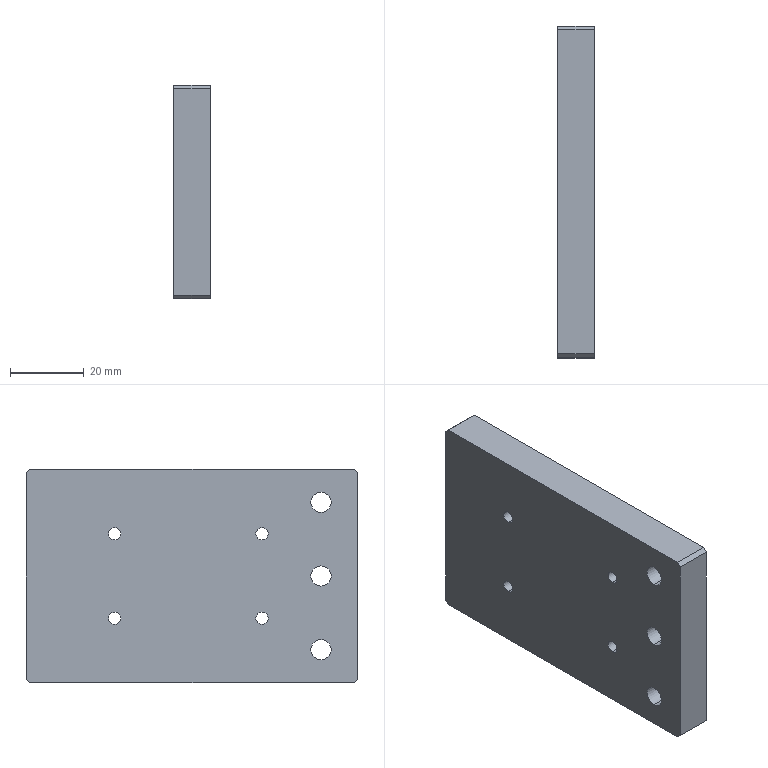Part | SolidWorks | features HoleWzd 2, Chamfer 1, Extrusion 1 | 1 solid | 33 faces | box 10 x 90 x 58 mm | volume 50238 mm3 | cylinder 20 | plane 13 | commonest cylinder face diameters 3.3 x8 5.5 x6 10 x6
STEP:
#1=CARTESIAN_POINT('',(4.6,-35.,25.));
#2=VERTEX_POINT('',#1);
#3=CARTESIAN_POINT('',(4.6,-35.,15.));
#4=VERTEX_POINT('',#3);
#5=CARTESIAN_POINT('',(4.6,-35.,20.));
#6=DIRECTION('',(1.,0.,0.));
#7=DIRECTION('',(0.,0.,-1.));
#8=AXIS2_PLACEMENT_3D('',#5,#6,#7);
#9=CIRCLE('',#8,5.);
#10=EDGE_CURVE('',#2,#4,#9,.T.);
#11=ORIENTED_EDGE('',*,*,#10,.F.);
#12=CARTESIAN_POINT('',(10.,-35.,25.));
#13=VERTEX_POINT('',#12);
#14=CARTESIAN_POINT('',(10.,-35.,25.));
#15=DIRECTION('',(1.,0.,0.));
#16=VECTOR('',#15,1000.);
#17=LINE('',#14,#16);
#18=EDGE_CURVE('',#2,#13,#17,.T.);
#19=ORIENTED_EDGE('',*,*,#18,.T.);
#20=CARTESIAN_POINT('',(10.,-35.,15.));
#21=VERTEX_POINT('',#20);
#22=CARTESIAN_POINT('',(10.,-35.,20.));
#23=DIRECTION('',(1.,0.,0.));
#24=DIRECTION('',(0.,0.,-1.));
#25=AXIS2_PLACEMENT_3D('',#22,#23,#24);
#26=CIRCLE('',#25,5.);
#27=EDGE_CURVE('',#13,#21,#26,.T.);
#28=ORIENTED_EDGE('',*,*,#27,.T.);
#29=CARTESIAN_POINT('',(10.,-35.,15.));
#30=DIRECTION('',(1.,0.,0.));
#31=VECTOR('',#30,1000.);
#32=LINE('',#29,#31);
#33=EDGE_CURVE('',#4,#21,#32,.T.);
#34=ORIENTED_EDGE('',*,*,#33,.F.);
#35=EDGE_LOOP('',(#11,#19,#28,#34));
#36=FACE_OUTER_BOUND('',#35,.T.);
#37=CARTESIAN_POINT('',(10.,-35.,20.));
#38=DIRECTION('',(1.,0.,0.));
#39=DIRECTION('',(0.,0.,-1.));
#40=AXIS2_PLACEMENT_3D('',#37,#38,#39);
#41=CYLINDRICAL_SURFACE('',#40,5.);
#42=ADVANCED_FACE('',(#36),#41,.F.);
#43=CARTESIAN_POINT('',(0.,-35.,22.75));
#44=VERTEX_POINT('',#43);
#45=CARTESIAN_POINT('',(0.,-35.,17.25));
#46=VERTEX_POINT('',#45);
#47=CARTESIAN_POINT('',(0.,-35.,20.));
#48=DIRECTION('',(1.,0.,0.));
#49=DIRECTION('',(0.,0.,-1.));
#50=AXIS2_PLACEMENT_3D('',#47,#48,#49);
#51=CIRCLE('',#50,2.75);
#52=EDGE_CURVE('',#44,#46,#51,.T.);
#53=ORIENTED_EDGE('',*,*,#52,.F.);
#54=CARTESIAN_POINT('',(4.6,-35.,22.75));
#55=VERTEX_POINT('',#54);
#56=CARTESIAN_POINT('',(10.,-35.,22.75));
#57=DIRECTION('',(1.,0.,0.));
#58=VECTOR('',#57,1000.);
#59=LINE('',#56,#58);
#60=EDGE_CURVE('',#44,#55,#59,.T.);
#61=ORIENTED_EDGE('',*,*,#60,.T.);
#62=CARTESIAN_POINT('',(4.6,-35.,17.25));
#63=VERTEX_POINT('',#62);
#64=CARTESIAN_POINT('',(4.6,-35.,20.));
#65=DIRECTION('',(1.,0.,0.));
#66=DIRECTION('',(0.,0.,-1.));
#67=AXIS2_PLACEMENT_3D('',#64,#65,#66);
#68=CIRCLE('',#67,2.75);
#69=EDGE_CURVE('',#55,#63,#68,.T.);
#70=ORIENTED_EDGE('',*,*,#69,.T.);
#71=CARTESIAN_POINT('',(10.,-35.,17.25));
#72=DIRECTION('',(1.,0.,0.));
#73=VECTOR('',#72,1000.);
#74=LINE('',#71,#73);
#75=EDGE_CURVE('',#46,#63,#74,.T.);
#76=ORIENTED_EDGE('',*,*,#75,.F.);
#77=EDGE_LOOP('',(#53,#61,#70,#76));
#78=FACE_OUTER_BOUND('',#77,.T.);
#79=CARTESIAN_POINT('',(10.,-35.,20.));
#80=DIRECTION('',(1.,0.,0.));
#81=DIRECTION('',(0.,0.,-1.));
#82=AXIS2_PLACEMENT_3D('',#79,#80,#81);
#83=CYLINDRICAL_SURFACE('',#82,2.75);
#84=ADVANCED_FACE('',(#78),#83,.F.);
#85=CARTESIAN_POINT('',(4.6,-35.,5.));
#86=VERTEX_POINT('',#85);
#87=CARTESIAN_POINT('',(4.6,-35.,-5.));
#88=VERTEX_POINT('',#87);
#89=CARTESIAN_POINT('',(4.6,-35.,0.));
#90=DIRECTION('',(1.,0.,0.));
#91=DIRECTION('',(0.,0.,-1.));
#92=AXIS2_PLACEMENT_3D('',#89,#90,#91);
#93=CIRCLE('',#92,5.);
#94=EDGE_CURVE('',#86,#88,#93,.T.);
#95=ORIENTED_EDGE('',*,*,#94,.F.);
#96=CARTESIAN_POINT('',(10.,-35.,5.));
#97=VERTEX_POINT('',#96);
#98=CARTESIAN_POINT('',(10.,-35.,5.));
#99=DIRECTION('',(1.,0.,0.));
#100=VECTOR('',#99,1000.);
#101=LINE('',#98,#100);
#102=EDGE_CURVE('',#86,#97,#101,.T.);
#103=ORIENTED_EDGE('',*,*,#102,.T.);
#104=CARTESIAN_POINT('',(10.,-35.,-5.));
#105=VERTEX_POINT('',#104);
#106=CARTESIAN_POINT('',(10.,-35.,0.));
#107=DIRECTION('',(1.,0.,0.));
#108=DIRECTION('',(0.,0.,-1.));
#109=AXIS2_PLACEMENT_3D('',#106,#107,#108);
#110=CIRCLE('',#109,5.);
#111=EDGE_CURVE('',#97,#105,#110,.T.);
#112=ORIENTED_EDGE('',*,*,#111,.T.);
#113=CARTESIAN_POINT('',(10.,-35.,-5.));
#114=DIRECTION('',(1.,0.,0.));
#115=VECTOR('',#114,1000.);
#116=LINE('',#113,#115);
#117=EDGE_CURVE('',#88,#105,#116,.T.);
#118=ORIENTED_EDGE('',*,*,#117,.F.);
#119=EDGE_LOOP('',(#95,#103,#112,#118));
#120=FACE_OUTER_BOUND('',#119,.T.);
#121=CARTESIAN_POINT('',(10.,-35.,0.));
#122=DIRECTION('',(1.,0.,0.));
#123=DIRECTION('',(0.,0.,-1.));
#124=AXIS2_PLACEMENT_3D('',#121,#122,#123);
#125=CYLINDRICAL_SURFACE('',#124,5.);
#126=ADVANCED_FACE('',(#120),#125,.F.);
#127=CARTESIAN_POINT('',(0.,-35.,2.75));
#128=VERTEX_POINT('',#127);
#129=CARTESIAN_POINT('',(0.,-35.,-2.75));
#130=VERTEX_POINT('',#129);
#131=CARTESIAN_POINT('',(0.,-35.,0.));
#132=DIRECTION('',(1.,0.,0.));
#133=DIRECTION('',(0.,0.,-1.));
#134=AXIS2_PLACEMENT_3D('',#131,#132,#133);
#135=CIRCLE('',#134,2.75);
#136=EDGE_CURVE('',#128,#130,#135,.T.);
#137=ORIENTED_EDGE('',*,*,#136,.F.);
#138=CARTESIAN_POINT('',(4.6,-35.,2.75));
#139=VERTEX_POINT('',#138);
#140=CARTESIAN_POINT('',(10.,-35.,2.75));
#141=DIRECTION('',(1.,0.,0.));
#142=VECTOR('',#141,1000.);
#143=LINE('',#140,#142);
#144=EDGE_CURVE('',#128,#139,#143,.T.);
#145=ORIENTED_EDGE('',*,*,#144,.T.);
#146=CARTESIAN_POINT('',(4.6,-35.,-2.75));
#147=VERTEX_POINT('',#146);
#148=CARTESIAN_POINT('',(4.6,-35.,0.));
#149=DIRECTION('',(1.,0.,0.));
#150=DIRECTION('',(0.,0.,-1.));
#151=AXIS2_PLACEMENT_3D('',#148,#149,#150);
#152=CIRCLE('',#151,2.75);
#153=EDGE_CURVE('',#139,#147,#152,.T.);
#154=ORIENTED_EDGE('',*,*,#153,.T.);
#155=CARTESIAN_POINT('',(10.,-35.,-2.75));
#156=DIRECTION('',(1.,0.,0.));
#157=VECTOR('',#156,1000.);
#158=LINE('',#155,#157);
#159=EDGE_CURVE('',#130,#147,#158,.T.);
#160=ORIENTED_EDGE('',*,*,#159,.F.);
#161=EDGE_LOOP('',(#137,#145,#154,#160));
#162=FACE_OUTER_BOUND('',#161,.T.);
#163=CARTESIAN_POINT('',(10.,-35.,0.));
#164=DIRECTION('',(1.,0.,0.));
#165=DIRECTION('',(0.,0.,-1.));
#166=AXIS2_PLACEMENT_3D('',#163,#164,#165);
#167=CYLINDRICAL_SURFACE('',#166,2.75);
#168=ADVANCED_FACE('',(#162),#167,.F.);
#169=CARTESIAN_POINT('',(4.6,-35.,-15.));
#170=VERTEX_POINT('',#169);
#171=CARTESIAN_POINT('',(4.6,-35.,-25.));
#172=VERTEX_POINT('',#171);
#173=CARTESIAN_POINT('',(4.6,-35.,-20.));
#174=DIRECTION('',(1.,0.,0.));
#175=DIRECTION('',(0.,0.,-1.));
#176=AXIS2_PLACEMENT_3D('',#173,#174,#175);
#177=CIRCLE('',#176,5.);
#178=EDGE_CURVE('',#170,#172,#177,.T.);
#179=ORIENTED_EDGE('',*,*,#178,.F.);
#180=CARTESIAN_POINT('',(10.,-35.,-15.));
#181=VERTEX_POINT('',#180);
#182=CARTESIAN_POINT('',(10.,-35.,-15.));
#183=DIRECTION('',(1.,0.,0.));
#184=VECTOR('',#183,1000.);
#185=LINE('',#182,#184);
#186=EDGE_CURVE('',#170,#181,#185,.T.);
#187=ORIENTED_EDGE('',*,*,#186,.T.);
#188=CARTESIAN_POINT('',(10.,-35.,-25.));
#189=VERTEX_POINT('',#188);
#190=CARTESIAN_POINT('',(10.,-35.,-20.));
#191=DIRECTION('',(1.,0.,0.));
#192=DIRECTION('',(0.,0.,-1.));
#193=AXIS2_PLACEMENT_3D('',#190,#191,#192);
#194=CIRCLE('',#193,5.);
#195=EDGE_CURVE('',#181,#189,#194,.T.);
#196=ORIENTED_EDGE('',*,*,#195,.T.);
#197=CARTESIAN_POINT('',(10.,-35.,-25.));
#198=DIRECTION('',(1.,0.,0.));
#199=VECTOR('',#198,1000.);
#200=LINE('',#197,#199);
#201=EDGE_CURVE('',#172,#189,#200,.T.);
#202=ORIENTED_EDGE('',*,*,#201,.F.);
#203=EDGE_LOOP('',(#179,#187,#196,#202));
#204=FACE_OUTER_BOUND('',#203,.T.);
#205=CARTESIAN_POINT('',(10.,-35.,-20.));
#206=DIRECTION('',(1.,0.,0.));
#207=DIRECTION('',(0.,0.,-1.));
#208=AXIS2_PLACEMENT_3D('',#205,#206,#207);
#209=CYLINDRICAL_SURFACE('',#208,5.);
#210=ADVANCED_FACE('',(#204),#209,.F.);
#211=CARTESIAN_POINT('',(0.,-35.,-17.25));
#212=VERTEX_POINT('',#211);
#213=CARTESIAN_POINT('',(0.,-35.,-22.75));
#214=VERTEX_POINT('',#213);
#215=CARTESIAN_POINT('',(0.,-35.,-20.));
#216=DIRECTION('',(1.,0.,0.));
#217=DIRECTION('',(0.,0.,-1.));
#218=AXIS2_PLACEMENT_3D('',#215,#216,#217);
#219=CIRCLE('',#218,2.75);
#220=EDGE_CURVE('',#212,#214,#219,.T.);
#221=ORIENTED_EDGE('',*,*,#220,.F.);
#222=CARTESIAN_POINT('',(4.6,-35.,-17.25));
#223=VERTEX_POINT('',#222);
#224=CARTESIAN_POINT('',(10.,-35.,-17.25));
#225=DIRECTION('',(1.,0.,0.));
#226=VECTOR('',#225,1000.);
#227=LINE('',#224,#226);
#228=EDGE_CURVE('',#212,#223,#227,.T.);
#229=ORIENTED_EDGE('',*,*,#228,.T.);
#230=CARTESIAN_POINT('',(4.6,-35.,-22.75));
#231=VERTEX_POINT('',#230);
#232=CARTESIAN_POINT('',(4.6,-35.,-20.));
#233=DIRECTION('',(1.,0.,0.));
#234=DIRECTION('',(0.,0.,-1.));
#235=AXIS2_PLACEMENT_3D('',#232,#233,#234);
#236=CIRCLE('',#235,2.75);
#237=EDGE_CURVE('',#223,#231,#236,.T.);
#238=ORIENTED_EDGE('',*,*,#237,.T.);
#239=CARTESIAN_POINT('',(10.,-35.,-22.75));
#240=DIRECTION('',(1.,0.,0.));
#241=VECTOR('',#240,1000.);
#242=LINE('',#239,#241);
#243=EDGE_CURVE('',#214,#231,#242,.T.);
#244=ORIENTED_EDGE('',*,*,#243,.F.);
#245=EDGE_LOOP('',(#221,#229,#238,#244));
#246=FACE_OUTER_BOUND('',#245,.T.);
#247=CARTESIAN_POINT('',(10.,-35.,-20.));
#248=DIRECTION('',(1.,0.,0.));
#249=DIRECTION('',(0.,0.,-1.));
#250=AXIS2_PLACEMENT_3D('',#247,#248,#249);
#251=CYLINDRICAL_SURFACE('',#250,2.75);
#252=ADVANCED_FACE('',(#246),#251,.F.);
#253=CARTESIAN_POINT('',(0.,21.,13.15));
#254=VERTEX_POINT('',#253);
#255=CARTESIAN_POINT('',(0.,21.,9.85));
#256=VERTEX_POINT('',#255);
#257=CARTESIAN_POINT('',(0.,21.,11.5));
#258=DIRECTION('',(1.,0.,0.));
#259=DIRECTION('',(0.,0.,-1.));
#260=AXIS2_PLACEMENT_3D('',#257,#258,#259);
#261=CIRCLE('',#260,1.65);
#262=EDGE_CURVE('',#254,#256,#261,.T.);
#263=ORIENTED_EDGE('',*,*,#262,.F.);
#264=CARTESIAN_POINT('',(10.,21.,13.15));
#265=VERTEX_POINT('',#264);
#266=CARTESIAN_POINT('',(10.,21.,13.15));
#267=DIRECTION('',(1.,0.,0.));
#268=VECTOR('',#267,1000.);
#269=LINE('',#266,#268);
#270=EDGE_CURVE('',#254,#265,#269,.T.);
#271=ORIENTED_EDGE('',*,*,#270,.T.);
#272=CARTESIAN_POINT('',(10.,21.,9.85));
#273=VERTEX_POINT('',#272);
#274=CARTESIAN_POINT('',(10.,21.,11.5));
#275=DIRECTION('',(1.,0.,0.));
#276=DIRECTION('',(0.,0.,-1.));
#277=AXIS2_PLACEMENT_3D('',#274,#275,#276);
#278=CIRCLE('',#277,1.65);
#279=EDGE_CURVE('',#265,#273,#278,.T.);
#280=ORIENTED_EDGE('',*,*,#279,.T.);
#281=CARTESIAN_POINT('',(10.,21.,9.85));
#282=DIRECTION('',(1.,0.,0.));
#283=VECTOR('',#282,1000.);
#284=LINE('',#281,#283);
#285=EDGE_CURVE('',#256,#273,#284,.T.);
#286=ORIENTED_EDGE('',*,*,#285,.F.);
#287=EDGE_LOOP('',(#263,#271,#280,#286));
#288=FACE_OUTER_BOUND('',#287,.T.);
#289=CARTESIAN_POINT('',(10.,21.,11.5));
#290=DIRECTION('',(1.,0.,0.));
#291=DIRECTION('',(0.,0.,-1.));
#292=AXIS2_PLACEMENT_3D('',#289,#290,#291);
#293=CYLINDRICAL_SURFACE('',#292,1.65);
#294=ADVANCED_FACE('',(#288),#293,.F.);
#295=CARTESIAN_POINT('',(0.,21.,-9.85));
#296=VERTEX_POINT('',#295);
#297=CARTESIAN_POINT('',(0.,21.,-13.15));
#298=VERTEX_POINT('',#297);
#299=CARTESIAN_POINT('',(0.,21.,-11.5));
#300=DIRECTION('',(1.,0.,0.));
#301=DIRECTION('',(0.,0.,-1.));
#302=AXIS2_PLACEMENT_3D('',#299,#300,#301);
#303=CIRCLE('',#302,1.65);
#304=EDGE_CURVE('',#296,#298,#303,.T.);
#305=ORIENTED_EDGE('',*,*,#304,.F.);
#306=CARTESIAN_POINT('',(10.,21.,-9.85));
#307=VERTEX_POINT('',#306);
#308=CARTESIAN_POINT('',(10.,21.,-9.85));
#309=DIRECTION('',(1.,0.,0.));
#310=VECTOR('',#309,1000.);
#311=LINE('',#308,#310);
#312=EDGE_CURVE('',#296,#307,#311,.T.);
#313=ORIENTED_EDGE('',*,*,#312,.T.);
#314=CARTESIAN_POINT('',(10.,21.,-13.15));
#315=VERTEX_POINT('',#314);
#316=CARTESIAN_POINT('',(10.,21.,-11.5));
#317=DIRECTION('',(1.,0.,0.));
#318=DIRECTION('',(0.,0.,-1.));
#319=AXIS2_PLACEMENT_3D('',#316,#317,#318);
#320=CIRCLE('',#319,1.65);
#321=EDGE_CURVE('',#307,#315,#320,.T.);
#322=ORIENTED_EDGE('',*,*,#321,.T.);
#323=CARTESIAN_POINT('',(10.,21.,-13.15));
#324=DIRECTION('',(1.,0.,0.));
#325=VECTOR('',#324,1000.);
#326=LINE('',#323,#325);
#327=EDGE_CURVE('',#298,#315,#326,.T.);
#328=ORIENTED_EDGE('',*,*,#327,.F.);
#329=EDGE_LOOP('',(#305,#313,#322,#328));
#330=FACE_OUTER_BOUND('',#329,.T.);
#331=CARTESIAN_POINT('',(10.,21.,-11.5));
#332=DIRECTION('',(1.,0.,0.));
#333=DIRECTION('',(0.,0.,-1.));
#334=AXIS2_PLACEMENT_3D('',#331,#332,#333);
#335=CYLINDRICAL_SURFACE('',#334,1.65);
#336=ADVANCED_FACE('',(#330),#335,.F.);
#337=CARTESIAN_POINT('',(0.,-19.,13.15));
#338=VERTEX_POINT('',#337);
#339=CARTESIAN_POINT('',(0.,-19.,9.85));
#340=VERTEX_POINT('',#339);
#341=CARTESIAN_POINT('',(0.,-19.,11.5));
#342=DIRECTION('',(1.,0.,0.));
#343=DIRECTION('',(0.,0.,-1.));
#344=AXIS2_PLACEMENT_3D('',#341,#342,#343);
#345=CIRCLE('',#344,1.65);
#346=EDGE_CURVE('',#338,#340,#345,.T.);
#347=ORIENTED_EDGE('',*,*,#346,.F.);
#348=CARTESIAN_POINT('',(10.,-19.,13.15));
#349=VERTEX_POINT('',#348);
#350=CARTESIAN_POINT('',(10.,-19.,13.15));
#351=DIRECTION('',(1.,0.,0.));
#352=VECTOR('',#351,1000.);
#353=LINE('',#350,#352);
#354=EDGE_CURVE('',#338,#349,#353,.T.);
#355=ORIENTED_EDGE('',*,*,#354,.T.);
#356=CARTESIAN_POINT('',(10.,-19.,9.85));
#357=VERTEX_POINT('',#356);
#358=CARTESIAN_POINT('',(10.,-19.,11.5));
#359=DIRECTION('',(1.,0.,0.));
#360=DIRECTION('',(0.,0.,-1.));
#361=AXIS2_PLACEMENT_3D('',#358,#359,#360);
#362=CIRCLE('',#361,1.65);
#363=EDGE_CURVE('',#349,#357,#362,.T.);
#364=ORIENTED_EDGE('',*,*,#363,.T.);
#365=CARTESIAN_POINT('',(10.,-19.,9.85));
#366=DIRECTION('',(1.,0.,0.));
#367=VECTOR('',#366,1000.);
#368=LINE('',#365,#367);
#369=EDGE_CURVE('',#340,#357,#368,.T.);
#370=ORIENTED_EDGE('',*,*,#369,.F.);
#371=EDGE_LOOP('',(#347,#355,#364,#370));
#372=FACE_OUTER_BOUND('',#371,.T.);
#373=CARTESIAN_POINT('',(10.,-19.,11.5));
#374=DIRECTION('',(1.,0.,0.));
#375=DIRECTION('',(0.,0.,-1.));
#376=AXIS2_PLACEMENT_3D('',#373,#374,#375);
#377=CYLINDRICAL_SURFACE('',#376,1.65);
#378=ADVANCED_FACE('',(#372),#377,.F.);
#379=CARTESIAN_POINT('',(0.,-19.,-9.85));
#380=VERTEX_POINT('',#379);
#381=CARTESIAN_POINT('',(0.,-19.,-13.15));
#382=VERTEX_POINT('',#381);
#383=CARTESIAN_POINT('',(0.,-19.,-11.5));
#384=DIRECTION('',(1.,0.,0.));
#385=DIRECTION('',(0.,0.,-1.));
#386=AXIS2_PLACEMENT_3D('',#383,#384,#385);
#387=CIRCLE('',#386,1.65);
#388=EDGE_CURVE('',#380,#382,#387,.T.);
#389=ORIENTED_EDGE('',*,*,#388,.F.);
#390=CARTESIAN_POINT('',(10.,-19.,-9.85));
#391=VERTEX_POINT('',#390);
#392=CARTESIAN_POINT('',(10.,-19.,-9.85));
#393=DIRECTION('',(1.,0.,0.));
#394=VECTOR('',#393,1000.);
#395=LINE('',#392,#394);
#396=EDGE_CURVE('',#380,#391,#395,.T.);
#397=ORIENTED_EDGE('',*,*,#396,.T.);
#398=CARTESIAN_POINT('',(10.,-19.,-13.15));
#399=VERTEX_POINT('',#398);
#400=CARTESIAN_POINT('',(10.,-19.,-11.5));
#401=DIRECTION('',(1.,0.,0.));
#402=DIRECTION('',(0.,0.,-1.));
#403=AXIS2_PLACEMENT_3D('',#400,#401,#402);
#404=CIRCLE('',#403,1.65);
#405=EDGE_CURVE('',#391,#399,#404,.T.);
#406=ORIENTED_EDGE('',*,*,#405,.T.);
#407=CARTESIAN_POINT('',(10.,-19.,-13.15));
#408=DIRECTION('',(1.,0.,0.));
#409=VECTOR('',#408,1000.);
#410=LINE('',#407,#409);
#411=EDGE_CURVE('',#382,#399,#410,.T.);
#412=ORIENTED_EDGE('',*,*,#411,.F.);
#413=EDGE_LOOP('',(#389,#397,#406,#412));
#414=FACE_OUTER_BOUND('',#413,.T.);
#415=CARTESIAN_POINT('',(10.,-19.,-11.5));
#416=DIRECTION('',(1.,0.,0.));
#417=DIRECTION('',(0.,0.,-1.));
#418=AXIS2_PLACEMENT_3D('',#415,#416,#417);
#419=CYLINDRICAL_SURFACE('',#418,1.65);
#420=ADVANCED_FACE('',(#414),#419,.F.);
#421=CARTESIAN_POINT('',(10.,-44.,-29.));
#422=VERTEX_POINT('',#421);
#423=CARTESIAN_POINT('',(10.,44.,-29.));
#424=VERTEX_POINT('',#423);
#425=CARTESIAN_POINT('',(10.,45.,-29.));
#426=DIRECTION('',(0.,1.,0.));
#427=VECTOR('',#426,1000.);
#428=LINE('',#425,#427);
#429=EDGE_CURVE('',#422,#424,#428,.T.);
#430=ORIENTED_EDGE('',*,*,#429,.F.);
#431=CARTESIAN_POINT('',(0.,-44.,-29.));
#432=VERTEX_POINT('',#431);
#433=CARTESIAN_POINT('',(10.,-44.,-29.));
#434=DIRECTION('',(-1.,0.,0.));
#435=VECTOR('',#434,1000.);
#436=LINE('',#433,#435);
#437=EDGE_CURVE('',#422,#432,#436,.T.);
#438=ORIENTED_EDGE('',*,*,#437,.T.);
#439=CARTESIAN_POINT('',(0.,44.,-29.));
#440=VERTEX_POINT('',#439);
#441=CARTESIAN_POINT('',(0.,45.,-29.));
#442=DIRECTION('',(0.,1.,0.));
#443=VECTOR('',#442,1000.);
#444=LINE('',#441,#443);
#445=EDGE_CURVE('',#432,#440,#444,.T.);
#446=ORIENTED_EDGE('',*,*,#445,.T.);
#447=CARTESIAN_POINT('',(10.,44.,-29.));
#448=DIRECTION('',(1.,0.,0.));
#449=VECTOR('',#448,1000.);
#450=LINE('',#447,#449);
#451=EDGE_CURVE('',#440,#424,#450,.T.);
#452=ORIENTED_EDGE('',*,*,#451,.T.);
#453=EDGE_LOOP('',(#430,#438,#446,#452));
#454=FACE_OUTER_BOUND('',#453,.T.);
#455=CARTESIAN_POINT('',(10.,45.,-29.));
#456=DIRECTION('',(0.,0.,1.));
#457=DIRECTION('',(0.,-1.,0.));
#458=AXIS2_PLACEMENT_3D('',#455,#456,#457);
#459=PLANE('',#458);
#460=ADVANCED_FACE('',(#454),#459,.F.);
#461=CARTESIAN_POINT('',(10.,45.,-28.));
#462=VERTEX_POINT('',#461);
#463=CARTESIAN_POINT('',(10.,45.,28.));
#464=VERTEX_POINT('',#463);
#465=CARTESIAN_POINT('',(10.,45.,29.));
#466=DIRECTION('',(0.,0.,1.));
#467=VECTOR('',#466,1000.);
#468=LINE('',#465,#467);
#469=EDGE_CURVE('',#462,#464,#468,.T.);
#470=ORIENTED_EDGE('',*,*,#469,.F.);
#471=CARTESIAN_POINT('',(0.,45.,-28.));
#472=VERTEX_POINT('',#471);
#473=CARTESIAN_POINT('',(10.,45.,-28.));
#474=DIRECTION('',(-1.,0.,0.));
#475=VECTOR('',#474,1000.);
#476=LINE('',#473,#475);
#477=EDGE_CURVE('',#462,#472,#476,.T.);
#478=ORIENTED_EDGE('',*,*,#477,.T.);
#479=CARTESIAN_POINT('',(0.,45.,28.));
#480=VERTEX_POINT('',#479);
#481=CARTESIAN_POINT('',(0.,45.,29.));
#482=DIRECTION('',(0.,0.,1.));
#483=VECTOR('',#482,1000.);
#484=LINE('',#481,#483);
#485=EDGE_CURVE('',#472,#480,#484,.T.);
#486=ORIENTED_EDGE('',*,*,#485,.T.);
#487=CARTESIAN_POINT('',(10.,45.,28.));
#488=DIRECTION('',(1.,0.,0.));
#489=VECTOR('',#488,1000.);
#490=LINE('',#487,#489);
#491=EDGE_CURVE('',#480,#464,#490,.T.);
#492=ORIENTED_EDGE('',*,*,#491,.T.);
#493=EDGE_LOOP('',(#470,#478,#486,#492));
#494=FACE_OUTER_BOUND('',#493,.T.);
#495=CARTESIAN_POINT('',(10.,45.,29.));
#496=DIRECTION('',(0.,-1.,0.));
#497=DIRECTION('',(0.,0.,-1.));
#498=AXIS2_PLACEMENT_3D('',#495,#496,#497);
#499=PLANE('',#498);
#500=ADVANCED_FACE('',(#494),#499,.F.);
#501=CARTESIAN_POINT('',(0.,44.,29.));
#502=VERTEX_POINT('',#501);
#503=CARTESIAN_POINT('',(0.,-44.,29.));
#504=VERTEX_POINT('',#503);
#505=CARTESIAN_POINT('',(0.,45.,29.));
#506=DIRECTION('',(0.,-1.,0.));
#507=VECTOR('',#506,1000.);
#508=LINE('',#505,#507);
#509=EDGE_CURVE('',#502,#504,#508,.T.);
#510=ORIENTED_EDGE('',*,*,#509,.T.);
#511=CARTESIAN_POINT('',(10.,-44.,29.));
#512=VERTEX_POINT('',#511);
#513=CARTESIAN_POINT('',(10.,-44.,29.));
#514=DIRECTION('',(1.,0.,0.));
#515=VECTOR('',#514,1000.);
#516=LINE('',#513,#515);
#517=EDGE_CURVE('',#504,#512,#516,.T.);
#518=ORIENTED_EDGE('',*,*,#517,.T.);
#519=CARTESIAN_POINT('',(10.,44.,29.));
#520=VERTEX_POINT('',#519);
#521=CARTESIAN_POINT('',(10.,45.,29.));
#522=DIRECTION('',(0.,-1.,0.));
#523=VECTOR('',#522,1000.);
#524=LINE('',#521,#523);
#525=EDGE_CURVE('',#520,#512,#524,.T.);
#526=ORIENTED_EDGE('',*,*,#525,.F.);
#527=CARTESIAN_POINT('',(10.,44.,29.));
#528=DIRECTION('',(-1.,0.,0.));
#529=VECTOR('',#528,1000.);
#530=LINE('',#527,#529);
#531=EDGE_CURVE('',#520,#502,#530,.T.);
#532=ORIENTED_EDGE('',*,*,#531,.T.);
#533=EDGE_LOOP('',(#510,#518,#526,#532));
#534=FACE_OUTER_BOUND('',#533,.T.);
#535=CARTESIAN_POINT('',(10.,45.,29.));
#536=DIRECTION('',(0.,0.,-1.));
#537=DIRECTION('',(0.,1.,0.));
#538=AXIS2_PLACEMENT_3D('',#535,#536,#537);
#539=PLANE('',#538);
#540=ADVANCED_FACE('',(#534),#539,.F.);
#541=CARTESIAN_POINT('',(0.,-45.,28.));
#542=VERTEX_POINT('',#541);
#543=CARTESIAN_POINT('',(0.,-45.,-28.));
#544=VERTEX_POINT('',#543);
#545=CARTESIAN_POINT('',(0.,-45.,29.));
#546=DIRECTION('',(0.,0.,-1.));
#547=VECTOR('',#546,1000.);
#548=LINE('',#545,#547);
#549=EDGE_CURVE('',#542,#544,#548,.T.);
#550=ORIENTED_EDGE('',*,*,#549,.T.);
#551=CARTESIAN_POINT('',(10.,-45.,-28.));
#552=VERTEX_POINT('',#551);
#553=CARTESIAN_POINT('',(10.,-45.,-28.));
#554=DIRECTION('',(1.,0.,0.));
#555=VECTOR('',#554,1000.);
#556=LINE('',#553,#555);
#557=EDGE_CURVE('',#544,#552,#556,.T.);
#558=ORIENTED_EDGE('',*,*,#557,.T.);
#559=CARTESIAN_POINT('',(10.,-45.,28.));
#560=VERTEX_POINT('',#559);
#561=CARTESIAN_POINT('',(10.,-45.,29.));
#562=DIRECTION('',(0.,0.,-1.));
#563=VECTOR('',#562,1000.);
#564=LINE('',#561,#563);
#565=EDGE_CURVE('',#560,#552,#564,.T.);
#566=ORIENTED_EDGE('',*,*,#565,.F.);
#567=CARTESIAN_POINT('',(10.,-45.,28.));
#568=DIRECTION('',(-1.,0.,0.));
#569=VECTOR('',#568,1000.);
#570=LINE('',#567,#569);
#571=EDGE_CURVE('',#560,#542,#570,.T.);
#572=ORIENTED_EDGE('',*,*,#571,.T.);
#573=EDGE_LOOP('',(#550,#558,#566,#572));
#574=FACE_OUTER_BOUND('',#573,.T.);
#575=CARTESIAN_POINT('',(10.,-45.,29.));
#576=DIRECTION('',(0.,1.,0.));
#577=DIRECTION('',(0.,0.,1.));
#578=AXIS2_PLACEMENT_3D('',#575,#576,#577);
#579=PLANE('',#578);
#580=ADVANCED_FACE('',(#574),#579,.F.);
#581=CARTESIAN_POINT('',(10.,-35.,20.));
#582=DIRECTION('',(1.,0.,0.));
#583=DIRECTION('',(0.,0.,-1.));
#584=AXIS2_PLACEMENT_3D('',#581,#582,#583);
#585=CIRCLE('',#584,5.);
#586=EDGE_CURVE('',#21,#13,#585,.T.);
#587=ORIENTED_EDGE('',*,*,#586,.F.);
#588=ORIENTED_EDGE('',*,*,#27,.F.);
#589=EDGE_LOOP('',(#587,#588));
#590=FACE_BOUND('',#589,.T.);
#591=CARTESIAN_POINT('',(10.,-35.,0.));
#592=DIRECTION('',(1.,0.,0.));
#593=DIRECTION('',(0.,0.,-1.));
#594=AXIS2_PLACEMENT_3D('',#591,#592,#593);
#595=CIRCLE('',#594,5.);
#596=EDGE_CURVE('',#105,#97,#595,.T.);
#597=ORIENTED_EDGE('',*,*,#596,.F.);
#598=ORIENTED_EDGE('',*,*,#111,.F.);
#599=EDGE_LOOP('',(#597,#598));
#600=FACE_BOUND('',#599,.T.);
#601=CARTESIAN_POINT('',(10.,-35.,-20.));
#602=DIRECTION('',(1.,0.,0.));
#603=DIRECTION('',(0.,0.,-1.));
#604=AXIS2_PLACEMENT_3D('',#601,#602,#603);
#605=CIRCLE('',#604,5.);
#606=EDGE_CURVE('',#189,#181,#605,.T.);
#607=ORIENTED_EDGE('',*,*,#606,.F.);
#608=ORIENTED_EDGE('',*,*,#195,.F.);
#609=EDGE_LOOP('',(#607,#608));
#610=FACE_BOUND('',#609,.T.);
#611=CARTESIAN_POINT('',(10.,21.,11.5));
#612=DIRECTION('',(1.,0.,0.));
#613=DIRECTION('',(0.,0.,-1.));
#614=AXIS2_PLACEMENT_3D('',#611,#612,#613);
#615=CIRCLE('',#614,1.65);
#616=EDGE_CURVE('',#273,#265,#615,.T.);
#617=ORIENTED_EDGE('',*,*,#616,.F.);
#618=ORIENTED_EDGE('',*,*,#279,.F.);
#619=EDGE_LOOP('',(#617,#618));
#620=FACE_BOUND('',#619,.T.);
#621=CARTESIAN_POINT('',(10.,21.,-11.5));
#622=DIRECTION('',(1.,0.,0.));
#623=DIRECTION('',(0.,0.,-1.));
#624=AXIS2_PLACEMENT_3D('',#621,#622,#623);
#625=CIRCLE('',#624,1.65);
#626=EDGE_CURVE('',#315,#307,#625,.T.);
#627=ORIENTED_EDGE('',*,*,#626,.F.);
#628=ORIENTED_EDGE('',*,*,#321,.F.);
#629=EDGE_LOOP('',(#627,#628));
#630=FACE_BOUND('',#629,.T.);
#631=CARTESIAN_POINT('',(10.,-19.,11.5));
#632=DIRECTION('',(1.,0.,0.));
#633=DIRECTION('',(0.,0.,-1.));
#634=AXIS2_PLACEMENT_3D('',#631,#632,#633);
#635=CIRCLE('',#634,1.65);
#636=EDGE_CURVE('',#357,#349,#635,.T.);
#637=ORIENTED_EDGE('',*,*,#636,.F.);
#638=ORIENTED_EDGE('',*,*,#363,.F.);
#639=EDGE_LOOP('',(#637,#638));
#640=FACE_BOUND('',#639,.T.);
#641=CARTESIAN_POINT('',(10.,-19.,-11.5));
#642=DIRECTION('',(1.,0.,0.));
#643=DIRECTION('',(0.,0.,-1.));
#644=AXIS2_PLACEMENT_3D('',#641,#642,#643);
#645=CIRCLE('',#644,1.65);
#646=EDGE_CURVE('',#399,#391,#645,.T.);
#647=ORIENTED_EDGE('',*,*,#646,.F.);
#648=ORIENTED_EDGE('',*,*,#405,.F.);
#649=EDGE_LOOP('',(#647,#648));
#650=FACE_BOUND('',#649,.T.);
#651=ORIENTED_EDGE('',*,*,#565,.T.);
#652=CARTESIAN_POINT('',(10.,-36.5,-36.5));
#653=DIRECTION('',(0.,0.7071,-0.7071));
#654=VECTOR('',#653,1000.);
#655=LINE('',#652,#654);
#656=EDGE_CURVE('',#552,#422,#655,.T.);
#657=ORIENTED_EDGE('',*,*,#656,.T.);
#658=ORIENTED_EDGE('',*,*,#429,.T.);
#659=CARTESIAN_POINT('',(10.,36.5,-36.5));
#660=DIRECTION('',(0.,0.7071,0.7071));
#661=VECTOR('',#660,1000.);
#662=LINE('',#659,#661);
#663=EDGE_CURVE('',#424,#462,#662,.T.);
#664=ORIENTED_EDGE('',*,*,#663,.T.);
#665=ORIENTED_EDGE('',*,*,#469,.T.);
#666=CARTESIAN_POINT('',(10.,36.5,36.5));
#667=DIRECTION('',(0.,-0.7071,0.7071));
#668=VECTOR('',#667,1000.);
#669=LINE('',#666,#668);
#670=EDGE_CURVE('',#464,#520,#669,.T.);
#671=ORIENTED_EDGE('',*,*,#670,.T.);
#672=ORIENTED_EDGE('',*,*,#525,.T.);
#673=CARTESIAN_POINT('',(10.,-36.5,36.5));
#674=DIRECTION('',(0.,-0.7071,-0.7071));
#675=VECTOR('',#674,1000.);
#676=LINE('',#673,#675);
#677=EDGE_CURVE('',#512,#560,#676,.T.);
#678=ORIENTED_EDGE('',*,*,#677,.T.);
#679=EDGE_LOOP('',(#651,#657,#658,#664,#665,#671,#672,#678));
#680=FACE_OUTER_BOUND('',#679,.T.);
#681=CARTESIAN_POINT('',(10.,0.,0.));
#682=DIRECTION('',(1.,0.,0.));
#683=DIRECTION('',(0.,0.,-1.));
#684=AXIS2_PLACEMENT_3D('',#681,#682,#683);
#685=PLANE('',#684);
#686=ADVANCED_FACE('',(#590,#600,#610,#620,#630,#640,#650,#680),#685,.T.);
#687=CARTESIAN_POINT('',(0.,-35.,20.));
#688=DIRECTION('',(1.,0.,0.));
#689=DIRECTION('',(0.,0.,-1.));
#690=AXIS2_PLACEMENT_3D('',#687,#688,#689);
#691=CIRCLE('',#690,2.75);
#692=EDGE_CURVE('',#46,#44,#691,.T.);
#693=ORIENTED_EDGE('',*,*,#692,.T.);
#694=ORIENTED_EDGE('',*,*,#52,.T.);
#695=EDGE_LOOP('',(#693,#694));
#696=FACE_BOUND('',#695,.T.);
#697=CARTESIAN_POINT('',(0.,-35.,0.));
#698=DIRECTION('',(1.,0.,0.));
#699=DIRECTION('',(0.,0.,-1.));
#700=AXIS2_PLACEMENT_3D('',#697,#698,#699);
#701=CIRCLE('',#700,2.75);
#702=EDGE_CURVE('',#130,#128,#701,.T.);
#703=ORIENTED_EDGE('',*,*,#702,.T.);
#704=ORIENTED_EDGE('',*,*,#136,.T.);
#705=EDGE_LOOP('',(#703,#704));
#706=FACE_BOUND('',#705,.T.);
#707=CARTESIAN_POINT('',(0.,-35.,-20.));
#708=DIRECTION('',(1.,0.,0.));
#709=DIRECTION('',(0.,0.,-1.));
#710=AXIS2_PLACEMENT_3D('',#707,#708,#709);
#711=CIRCLE('',#710,2.75);
#712=EDGE_CURVE('',#214,#212,#711,.T.);
#713=ORIENTED_EDGE('',*,*,#712,.T.);
#714=ORIENTED_EDGE('',*,*,#220,.T.);
#715=EDGE_LOOP('',(#713,#714));
#716=FACE_BOUND('',#715,.T.);
#717=CARTESIAN_POINT('',(0.,21.,11.5));
#718=DIRECTION('',(1.,0.,0.));
#719=DIRECTION('',(0.,0.,-1.));
#720=AXIS2_PLACEMENT_3D('',#717,#718,#719);
#721=CIRCLE('',#720,1.65);
#722=EDGE_CURVE('',#256,#254,#721,.T.);
#723=ORIENTED_EDGE('',*,*,#722,.T.);
#724=ORIENTED_EDGE('',*,*,#262,.T.);
#725=EDGE_LOOP('',(#723,#724));
#726=FACE_BOUND('',#725,.T.);
#727=CARTESIAN_POINT('',(0.,21.,-11.5));
#728=DIRECTION('',(1.,0.,0.));
#729=DIRECTION('',(0.,0.,-1.));
#730=AXIS2_PLACEMENT_3D('',#727,#728,#729);
#731=CIRCLE('',#730,1.65);
#732=EDGE_CURVE('',#298,#296,#731,.T.);
#733=ORIENTED_EDGE('',*,*,#732,.T.);
#734=ORIENTED_EDGE('',*,*,#304,.T.);
#735=EDGE_LOOP('',(#733,#734));
#736=FACE_BOUND('',#735,.T.);
#737=CARTESIAN_POINT('',(0.,-19.,11.5));
#738=DIRECTION('',(1.,0.,0.));
#739=DIRECTION('',(0.,0.,-1.));
#740=AXIS2_PLACEMENT_3D('',#737,#738,#739);
#741=CIRCLE('',#740,1.65);
#742=EDGE_CURVE('',#340,#338,#741,.T.);
#743=ORIENTED_EDGE('',*,*,#742,.T.);
#744=ORIENTED_EDGE('',*,*,#346,.T.);
#745=EDGE_LOOP('',(#743,#744));
#746=FACE_BOUND('',#745,.T.);
#747=CARTESIAN_POINT('',(0.,-19.,-11.5));
#748=DIRECTION('',(1.,0.,0.));
#749=DIRECTION('',(0.,0.,-1.));
#750=AXIS2_PLACEMENT_3D('',#747,#748,#749);
#751=CIRCLE('',#750,1.65);
#752=EDGE_CURVE('',#382,#380,#751,.T.);
#753=ORIENTED_EDGE('',*,*,#752,.T.);
#754=ORIENTED_EDGE('',*,*,#388,.T.);
#755=EDGE_LOOP('',(#753,#754));
#756=FACE_BOUND('',#755,.T.);
#757=ORIENTED_EDGE('',*,*,#445,.F.);
#758=CARTESIAN_POINT('',(0.,-44.,-29.));
#759=DIRECTION('',(0.,-0.7071,0.7071));
#760=VECTOR('',#759,1000.);
#761=LINE('',#758,#760);
#762=EDGE_CURVE('',#432,#544,#761,.T.);
#763=ORIENTED_EDGE('',*,*,#762,.T.);
#764=ORIENTED_EDGE('',*,*,#549,.F.);
#765=CARTESIAN_POINT('',(0.,-45.,28.));
#766=DIRECTION('',(0.,0.7071,0.7071));
#767=VECTOR('',#766,1000.);
#768=LINE('',#765,#767);
#769=EDGE_CURVE('',#542,#504,#768,.T.);
#770=ORIENTED_EDGE('',*,*,#769,.T.);
#771=ORIENTED_EDGE('',*,*,#509,.F.);
#772=CARTESIAN_POINT('',(0.,44.,29.));
#773=DIRECTION('',(0.,0.7071,-0.7071));
#774=VECTOR('',#773,1000.);
#775=LINE('',#772,#774);
#776=EDGE_CURVE('',#502,#480,#775,.T.);
#777=ORIENTED_EDGE('',*,*,#776,.T.);
#778=ORIENTED_EDGE('',*,*,#485,.F.);
#779=CARTESIAN_POINT('',(0.,45.,-28.));
#780=DIRECTION('',(0.,-0.7071,-0.7071));
#781=VECTOR('',#780,1000.);
#782=LINE('',#779,#781);
#783=EDGE_CURVE('',#472,#440,#782,.T.);
#784=ORIENTED_EDGE('',*,*,#783,.T.);
#785=EDGE_LOOP('',(#757,#763,#764,#770,#771,#777,#778,#784));
#786=FACE_OUTER_BOUND('',#785,.T.);
#787=CARTESIAN_POINT('',(0.,0.,0.));
#788=DIRECTION('',(1.,0.,0.));
#789=DIRECTION('',(0.,0.,-1.));
#790=AXIS2_PLACEMENT_3D('',#787,#788,#789);
#791=PLANE('',#790);
#792=ADVANCED_FACE('',(#696,#706,#716,#726,#736,#746,#756,#786),#791,.F.);
#793=ORIENTED_EDGE('',*,*,#396,.F.);
#794=ORIENTED_EDGE('',*,*,#752,.F.);
#795=ORIENTED_EDGE('',*,*,#411,.T.);
#796=ORIENTED_EDGE('',*,*,#646,.T.);
#797=EDGE_LOOP('',(#793,#794,#795,#796));
#798=FACE_OUTER_BOUND('',#797,.T.);
#799=CARTESIAN_POINT('',(10.,-19.,-11.5));
#800=DIRECTION('',(1.,0.,0.));
#801=DIRECTION('',(0.,0.,-1.));
#802=AXIS2_PLACEMENT_3D('',#799,#800,#801);
#803=CYLINDRICAL_SURFACE('',#802,1.65);
#804=ADVANCED_FACE('',(#798),#803,.F.);
#805=ORIENTED_EDGE('',*,*,#354,.F.);
#806=ORIENTED_EDGE('',*,*,#742,.F.);
#807=ORIENTED_EDGE('',*,*,#369,.T.);
#808=ORIENTED_EDGE('',*,*,#636,.T.);
#809=EDGE_LOOP('',(#805,#806,#807,#808));
#810=FACE_OUTER_BOUND('',#809,.T.);
#811=CARTESIAN_POINT('',(10.,-19.,11.5));
#812=DIRECTION('',(1.,0.,0.));
#813=DIRECTION('',(0.,0.,-1.));
#814=AXIS2_PLACEMENT_3D('',#811,#812,#813);
#815=CYLINDRICAL_SURFACE('',#814,1.65);
#816=ADVANCED_FACE('',(#810),#815,.F.);
#817=ORIENTED_EDGE('',*,*,#312,.F.);
#818=ORIENTED_EDGE('',*,*,#732,.F.);
#819=ORIENTED_EDGE('',*,*,#327,.T.);
#820=ORIENTED_EDGE('',*,*,#626,.T.);
#821=EDGE_LOOP('',(#817,#818,#819,#820));
#822=FACE_OUTER_BOUND('',#821,.T.);
#823=CARTESIAN_POINT('',(10.,21.,-11.5));
#824=DIRECTION('',(1.,0.,0.));
#825=DIRECTION('',(0.,0.,-1.));
#826=AXIS2_PLACEMENT_3D('',#823,#824,#825);
#827=CYLINDRICAL_SURFACE('',#826,1.65);
#828=ADVANCED_FACE('',(#822),#827,.F.);
#829=ORIENTED_EDGE('',*,*,#270,.F.);
#830=ORIENTED_EDGE('',*,*,#722,.F.);
#831=ORIENTED_EDGE('',*,*,#285,.T.);
#832=ORIENTED_EDGE('',*,*,#616,.T.);
#833=EDGE_LOOP('',(#829,#830,#831,#832));
#834=FACE_OUTER_BOUND('',#833,.T.);
#835=CARTESIAN_POINT('',(10.,21.,11.5));
#836=DIRECTION('',(1.,0.,0.));
#837=DIRECTION('',(0.,0.,-1.));
#838=AXIS2_PLACEMENT_3D('',#835,#836,#837);
#839=CYLINDRICAL_SURFACE('',#838,1.65);
#840=ADVANCED_FACE('',(#834),#839,.F.);
#841=ORIENTED_EDGE('',*,*,#228,.F.);
#842=ORIENTED_EDGE('',*,*,#712,.F.);
#843=ORIENTED_EDGE('',*,*,#243,.T.);
#844=CARTESIAN_POINT('',(4.6,-35.,-20.));
#845=DIRECTION('',(1.,0.,0.));
#846=DIRECTION('',(0.,0.,-1.));
#847=AXIS2_PLACEMENT_3D('',#844,#845,#846);
#848=CIRCLE('',#847,2.75);
#849=EDGE_CURVE('',#231,#223,#848,.T.);
#850=ORIENTED_EDGE('',*,*,#849,.T.);
#851=EDGE_LOOP('',(#841,#842,#843,#850));
#852=FACE_OUTER_BOUND('',#851,.T.);
#853=CARTESIAN_POINT('',(10.,-35.,-20.));
#854=DIRECTION('',(1.,0.,0.));
#855=DIRECTION('',(0.,0.,-1.));
#856=AXIS2_PLACEMENT_3D('',#853,#854,#855);
#857=CYLINDRICAL_SURFACE('',#856,2.75);
#858=ADVANCED_FACE('',(#852),#857,.F.);
#859=ORIENTED_EDGE('',*,*,#849,.F.);
#860=ORIENTED_EDGE('',*,*,#237,.F.);
#861=EDGE_LOOP('',(#859,#860));
#862=FACE_BOUND('',#861,.T.);
#863=CARTESIAN_POINT('',(4.6,-35.,-20.));
#864=DIRECTION('',(1.,0.,0.));
#865=DIRECTION('',(0.,0.,-1.));
#866=AXIS2_PLACEMENT_3D('',#863,#864,#865);
#867=CIRCLE('',#866,5.);
#868=EDGE_CURVE('',#172,#170,#867,.T.);
#869=ORIENTED_EDGE('',*,*,#868,.T.);
#870=ORIENTED_EDGE('',*,*,#178,.T.);
#871=EDGE_LOOP('',(#869,#870));
#872=FACE_OUTER_BOUND('',#871,.T.);
#873=CARTESIAN_POINT('',(4.6,-32.25,-20.));
#874=DIRECTION('',(-1.,0.,0.));
#875=DIRECTION('',(0.,0.,1.));
#876=AXIS2_PLACEMENT_3D('',#873,#874,#875);
#877=PLANE('',#876);
#878=ADVANCED_FACE('',(#862,#872),#877,.F.);
#879=ORIENTED_EDGE('',*,*,#186,.F.);
#880=ORIENTED_EDGE('',*,*,#868,.F.);
#881=ORIENTED_EDGE('',*,*,#201,.T.);
#882=ORIENTED_EDGE('',*,*,#606,.T.);
#883=EDGE_LOOP('',(#879,#880,#881,#882));
#884=FACE_OUTER_BOUND('',#883,.T.);
#885=CARTESIAN_POINT('',(10.,-35.,-20.));
#886=DIRECTION('',(1.,0.,0.));
#887=DIRECTION('',(0.,0.,-1.));
#888=AXIS2_PLACEMENT_3D('',#885,#886,#887);
#889=CYLINDRICAL_SURFACE('',#888,5.);
#890=ADVANCED_FACE('',(#884),#889,.F.);
#891=ORIENTED_EDGE('',*,*,#144,.F.);
#892=ORIENTED_EDGE('',*,*,#702,.F.);
#893=ORIENTED_EDGE('',*,*,#159,.T.);
#894=CARTESIAN_POINT('',(4.6,-35.,0.));
#895=DIRECTION('',(1.,0.,0.));
#896=DIRECTION('',(0.,0.,-1.));
#897=AXIS2_PLACEMENT_3D('',#894,#895,#896);
#898=CIRCLE('',#897,2.75);
#899=EDGE_CURVE('',#147,#139,#898,.T.);
#900=ORIENTED_EDGE('',*,*,#899,.T.);
#901=EDGE_LOOP('',(#891,#892,#893,#900));
#902=FACE_OUTER_BOUND('',#901,.T.);
#903=CARTESIAN_POINT('',(10.,-35.,0.));
#904=DIRECTION('',(1.,0.,0.));
#905=DIRECTION('',(0.,0.,-1.));
#906=AXIS2_PLACEMENT_3D('',#903,#904,#905);
#907=CYLINDRICAL_SURFACE('',#906,2.75);
#908=ADVANCED_FACE('',(#902),#907,.F.);
#909=ORIENTED_EDGE('',*,*,#899,.F.);
#910=ORIENTED_EDGE('',*,*,#153,.F.);
#911=EDGE_LOOP('',(#909,#910));
#912=FACE_BOUND('',#911,.T.);
#913=CARTESIAN_POINT('',(4.6,-35.,0.));
#914=DIRECTION('',(1.,0.,0.));
#915=DIRECTION('',(0.,0.,-1.));
#916=AXIS2_PLACEMENT_3D('',#913,#914,#915);
#917=CIRCLE('',#916,5.);
#918=EDGE_CURVE('',#88,#86,#917,.T.);
#919=ORIENTED_EDGE('',*,*,#918,.T.);
#920=ORIENTED_EDGE('',*,*,#94,.T.);
#921=EDGE_LOOP('',(#919,#920));
#922=FACE_OUTER_BOUND('',#921,.T.);
#923=CARTESIAN_POINT('',(4.6,-32.25,0.));
#924=DIRECTION('',(-1.,0.,0.));
#925=DIRECTION('',(0.,0.,1.));
#926=AXIS2_PLACEMENT_3D('',#923,#924,#925);
#927=PLANE('',#926);
#928=ADVANCED_FACE('',(#912,#922),#927,.F.);
#929=ORIENTED_EDGE('',*,*,#102,.F.);
#930=ORIENTED_EDGE('',*,*,#918,.F.);
#931=ORIENTED_EDGE('',*,*,#117,.T.);
#932=ORIENTED_EDGE('',*,*,#596,.T.);
#933=EDGE_LOOP('',(#929,#930,#931,#932));
#934=FACE_OUTER_BOUND('',#933,.T.);
#935=CARTESIAN_POINT('',(10.,-35.,0.));
#936=DIRECTION('',(1.,0.,0.));
#937=DIRECTION('',(0.,0.,-1.));
#938=AXIS2_PLACEMENT_3D('',#935,#936,#937);
#939=CYLINDRICAL_SURFACE('',#938,5.);
#940=ADVANCED_FACE('',(#934),#939,.F.);
#941=ORIENTED_EDGE('',*,*,#60,.F.);
#942=ORIENTED_EDGE('',*,*,#692,.F.);
#943=ORIENTED_EDGE('',*,*,#75,.T.);
#944=CARTESIAN_POINT('',(4.6,-35.,20.));
#945=DIRECTION('',(1.,0.,0.));
#946=DIRECTION('',(0.,0.,-1.));
#947=AXIS2_PLACEMENT_3D('',#944,#945,#946);
#948=CIRCLE('',#947,2.75);
#949=EDGE_CURVE('',#63,#55,#948,.T.);
#950=ORIENTED_EDGE('',*,*,#949,.T.);
#951=EDGE_LOOP('',(#941,#942,#943,#950));
#952=FACE_OUTER_BOUND('',#951,.T.);
#953=CARTESIAN_POINT('',(10.,-35.,20.));
#954=DIRECTION('',(1.,0.,0.));
#955=DIRECTION('',(0.,0.,-1.));
#956=AXIS2_PLACEMENT_3D('',#953,#954,#955);
#957=CYLINDRICAL_SURFACE('',#956,2.75);
#958=ADVANCED_FACE('',(#952),#957,.F.);
#959=ORIENTED_EDGE('',*,*,#949,.F.);
#960=ORIENTED_EDGE('',*,*,#69,.F.);
#961=EDGE_LOOP('',(#959,#960));
#962=FACE_BOUND('',#961,.T.);
#963=CARTESIAN_POINT('',(4.6,-35.,20.));
#964=DIRECTION('',(1.,0.,0.));
#965=DIRECTION('',(0.,0.,-1.));
#966=AXIS2_PLACEMENT_3D('',#963,#964,#965);
#967=CIRCLE('',#966,5.);
#968=EDGE_CURVE('',#4,#2,#967,.T.);
#969=ORIENTED_EDGE('',*,*,#968,.T.);
#970=ORIENTED_EDGE('',*,*,#10,.T.);
#971=EDGE_LOOP('',(#969,#970));
#972=FACE_OUTER_BOUND('',#971,.T.);
#973=CARTESIAN_POINT('',(4.6,-32.25,20.));
#974=DIRECTION('',(-1.,0.,0.));
#975=DIRECTION('',(0.,0.,1.));
#976=AXIS2_PLACEMENT_3D('',#973,#974,#975);
#977=PLANE('',#976);
#978=ADVANCED_FACE('',(#962,#972),#977,.F.);
#979=ORIENTED_EDGE('',*,*,#18,.F.);
#980=ORIENTED_EDGE('',*,*,#968,.F.);
#981=ORIENTED_EDGE('',*,*,#33,.T.);
#982=ORIENTED_EDGE('',*,*,#586,.T.);
#983=EDGE_LOOP('',(#979,#980,#981,#982));
#984=FACE_OUTER_BOUND('',#983,.T.);
#985=CARTESIAN_POINT('',(10.,-35.,20.));
#986=DIRECTION('',(1.,0.,0.));
#987=DIRECTION('',(0.,0.,-1.));
#988=AXIS2_PLACEMENT_3D('',#985,#986,#987);
#989=CYLINDRICAL_SURFACE('',#988,5.);
#990=ADVANCED_FACE('',(#984),#989,.F.);
#991=ORIENTED_EDGE('',*,*,#656,.F.);
#992=ORIENTED_EDGE('',*,*,#557,.F.);
#993=ORIENTED_EDGE('',*,*,#762,.F.);
#994=ORIENTED_EDGE('',*,*,#437,.F.);
#995=EDGE_LOOP('',(#991,#992,#993,#994));
#996=FACE_OUTER_BOUND('',#995,.T.);
#997=CARTESIAN_POINT('',(10.,-44.,-29.));
#998=DIRECTION('',(0.,0.7071,0.7071));
#999=DIRECTION('',(-1.,0.,0.));
#1000=AXIS2_PLACEMENT_3D('',#997,#998,#999);
#1001=PLANE('',#1000);
#1002=ADVANCED_FACE('',(#996),#1001,.F.);
#1003=ORIENTED_EDGE('',*,*,#677,.F.);
#1004=ORIENTED_EDGE('',*,*,#517,.F.);
#1005=ORIENTED_EDGE('',*,*,#769,.F.);
#1006=ORIENTED_EDGE('',*,*,#571,.F.);
#1007=EDGE_LOOP('',(#1003,#1004,#1005,#1006));
#1008=FACE_OUTER_BOUND('',#1007,.T.);
#1009=CARTESIAN_POINT('',(10.,-45.,28.));
#1010=DIRECTION('',(0.,0.7071,-0.7071));
#1011=DIRECTION('',(-1.,0.,0.));
#1012=AXIS2_PLACEMENT_3D('',#1009,#1010,#1011);
#1013=PLANE('',#1012);
#1014=ADVANCED_FACE('',(#1008),#1013,.F.);
#1015=ORIENTED_EDGE('',*,*,#663,.F.);
#1016=ORIENTED_EDGE('',*,*,#451,.F.);
#1017=ORIENTED_EDGE('',*,*,#783,.F.);
#1018=ORIENTED_EDGE('',*,*,#477,.F.);
#1019=EDGE_LOOP('',(#1015,#1016,#1017,#1018));
#1020=FACE_OUTER_BOUND('',#1019,.T.);
#1021=CARTESIAN_POINT('',(10.,45.,-28.));
#1022=DIRECTION('',(0.,-0.7071,0.7071));
#1023=DIRECTION('',(-1.,0.,0.));
#1024=AXIS2_PLACEMENT_3D('',#1021,#1022,#1023);
#1025=PLANE('',#1024);
#1026=ADVANCED_FACE('',(#1020),#1025,.F.);
#1027=ORIENTED_EDGE('',*,*,#670,.F.);
#1028=ORIENTED_EDGE('',*,*,#491,.F.);
#1029=ORIENTED_EDGE('',*,*,#776,.F.);
#1030=ORIENTED_EDGE('',*,*,#531,.F.);
#1031=EDGE_LOOP('',(#1027,#1028,#1029,#1030));
#1032=FACE_OUTER_BOUND('',#1031,.T.);
#1033=CARTESIAN_POINT('',(10.,44.,29.));
#1034=DIRECTION('',(0.,-0.7071,-0.7071));
#1035=DIRECTION('',(-1.,0.,0.));
#1036=AXIS2_PLACEMENT_3D('',#1033,#1034,#1035);
#1037=PLANE('',#1036);
#1038=ADVANCED_FACE('',(#1032),#1037,.F.);
#1039=CLOSED_SHELL('',(#42,#84,#126,#168,#210,#252,#294,#336,#378,#420,#460,#500,#540,#580,#686,#792,#804,#816,#828,#840,#858,#878,#890,#908,#928,#940,#958,#978,#990,#1002,#1014,#1026,#1038));
#1040=MANIFOLD_SOLID_BREP('',#1039);
#1041=CARTESIAN_POINT('',(0.,0.,0.));
#1042=DIRECTION('',(0.,0.,1.));
#1043=DIRECTION('',(1.,0.,0.));
#1044=AXIS2_PLACEMENT_3D('',#1041,#1042,#1043);
#1045=(LENGTH_UNIT()NAMED_UNIT(*)SI_UNIT(.MILLI.,.METRE.));
#1046=UNCERTAINTY_MEASURE_WITH_UNIT(LENGTH_MEASURE(0.00001),#1045,'','');
#1047=(NAMED_UNIT(*)PLANE_ANGLE_UNIT()SI_UNIT($,.RADIAN.));
#1048=(NAMED_UNIT(*)SI_UNIT($,.STERADIAN.)SOLID_ANGLE_UNIT());
#1049=(GEOMETRIC_REPRESENTATION_CONTEXT(3)GLOBAL_UNCERTAINTY_ASSIGNED_CONTEXT((#1046))GLOBAL_UNIT_ASSIGNED_CONTEXT((#1045,#1047,#1048))REPRESENTATION_CONTEXT('',''));
#1050=ADVANCED_BREP_SHAPE_REPRESENTATION('',(#1040,#1044),#1049);